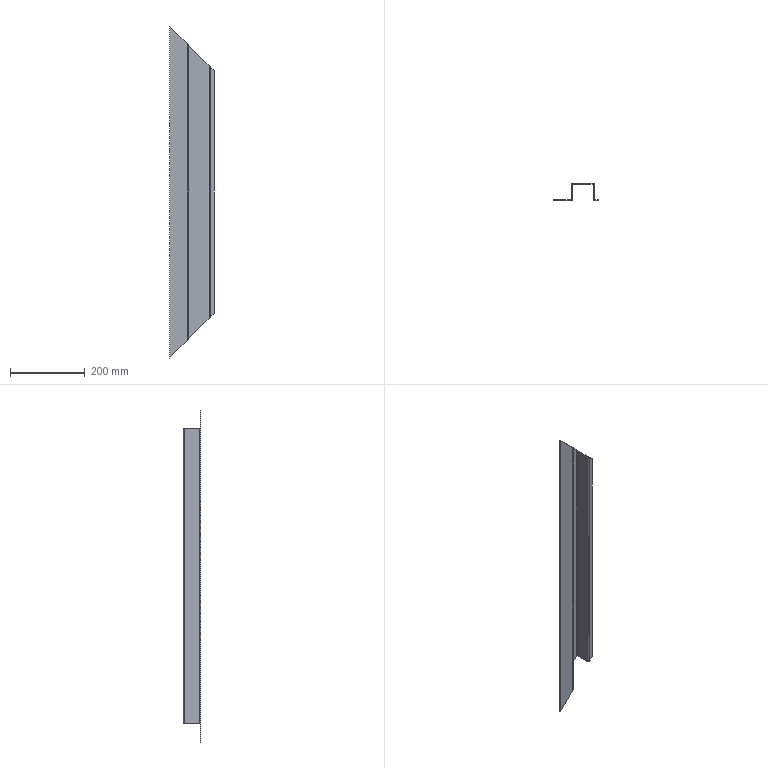Part | STEP file | 750038413 | 1 solid | 38 faces | box 120 x 46.5 x 888 mm | volume 232487 mm3 | plane 22 | cylinder 8 | spline 8 | commonest cylinder face diameters 3 x4 6 x4
STEP:
#1=CARTESIAN_POINT('',(-120.,-1.5,444.));
#2=VERTEX_POINT('',#1);
#3=CARTESIAN_POINT('',(-120.,-1.5,-444.));
#4=VERTEX_POINT('',#3);
#5=CARTESIAN_POINT('',(-120.,-1.5,444.));
#6=DIRECTION('',(0.,0.,-1.));
#7=VECTOR('',#6,1000.);
#8=LINE('',#5,#7);
#9=EDGE_CURVE('',#2,#4,#8,.T.);
#10=ORIENTED_EDGE('',*,*,#9,.T.);
#11=CARTESIAN_POINT('',(-73.,-1.5,-397.));
#12=VERTEX_POINT('',#11);
#13=CARTESIAN_POINT('',(-120.,-1.5,-444.));
#14=DIRECTION('',(0.7071,0.,0.7071));
#15=VECTOR('',#14,1000.);
#16=LINE('',#13,#15);
#17=EDGE_CURVE('',#4,#12,#16,.T.);
#18=ORIENTED_EDGE('',*,*,#17,.T.);
#19=CARTESIAN_POINT('',(-73.,-1.5,397.));
#20=VERTEX_POINT('',#19);
#21=CARTESIAN_POINT('',(-73.,-1.5,444.));
#22=DIRECTION('',(0.,0.,1.));
#23=VECTOR('',#22,1000.);
#24=LINE('',#21,#23);
#25=EDGE_CURVE('',#12,#20,#24,.T.);
#26=ORIENTED_EDGE('',*,*,#25,.T.);
#27=CARTESIAN_POINT('',(-73.,-1.5,397.));
#28=DIRECTION('',(-0.7071,0.,0.7071));
#29=VECTOR('',#28,1000.);
#30=LINE('',#27,#29);
#31=EDGE_CURVE('',#20,#2,#30,.T.);
#32=ORIENTED_EDGE('',*,*,#31,.T.);
#33=EDGE_LOOP('',(#10,#18,#26,#32));
#34=FACE_OUTER_BOUND('',#33,.T.);
#35=CARTESIAN_POINT('',(-71.5,-1.5,444.));
#36=DIRECTION('',(0.,-1.,0.));
#37=DIRECTION('',(1.,0.,0.));
#38=AXIS2_PLACEMENT_3D('',#35,#36,#37);
#39=PLANE('',#38);
#40=ADVANCED_FACE('',(#34),#39,.T.);
#41=CARTESIAN_POINT('',(-73.,0.,-397.));
#42=VERTEX_POINT('',#41);
#43=CARTESIAN_POINT('',(-73.,-0.75,-397.));
#44=DIRECTION('',(0.,-1.,0.));
#45=VECTOR('',#44,1000.);
#46=LINE('',#43,#45);
#47=EDGE_CURVE('',#42,#12,#46,.T.);
#48=ORIENTED_EDGE('',*,*,#47,.T.);
#49=ORIENTED_EDGE('',*,*,#17,.F.);
#50=CARTESIAN_POINT('',(-120.,0.,-444.));
#51=VERTEX_POINT('',#50);
#52=CARTESIAN_POINT('',(-120.,0.,-444.));
#53=DIRECTION('',(0.,1.,0.));
#54=VECTOR('',#53,1000.);
#55=LINE('',#52,#54);
#56=EDGE_CURVE('',#4,#51,#55,.T.);
#57=ORIENTED_EDGE('',*,*,#56,.T.);
#58=CARTESIAN_POINT('',(348.25,0.,24.25));
#59=DIRECTION('',(0.7071,0.,0.7071));
#60=VECTOR('',#59,1000.);
#61=LINE('',#58,#60);
#62=EDGE_CURVE('',#51,#42,#61,.T.);
#63=ORIENTED_EDGE('',*,*,#62,.T.);
#64=EDGE_LOOP('',(#48,#49,#57,#63));
#65=FACE_OUTER_BOUND('',#64,.T.);
#66=CARTESIAN_POINT('',(348.25,0.,24.25));
#67=DIRECTION('',(0.7071,0.,-0.7071));
#68=DIRECTION('',(-0.7071,0.,-0.7071));
#69=AXIS2_PLACEMENT_3D('',#66,#67,#68);
#70=PLANE('',#69);
#71=ADVANCED_FACE('',(#65),#70,.T.);
#72=ORIENTED_EDGE('',*,*,#56,.F.);
#73=ORIENTED_EDGE('',*,*,#9,.F.);
#74=CARTESIAN_POINT('',(-120.,0.,444.));
#75=VERTEX_POINT('',#74);
#76=CARTESIAN_POINT('',(-120.,0.,444.));
#77=DIRECTION('',(0.,1.,0.));
#78=VECTOR('',#77,1000.);
#79=LINE('',#76,#78);
#80=EDGE_CURVE('',#2,#75,#79,.T.);
#81=ORIENTED_EDGE('',*,*,#80,.T.);
#82=CARTESIAN_POINT('',(-120.,0.,444.));
#83=DIRECTION('',(0.,0.,-1.));
#84=VECTOR('',#83,1000.);
#85=LINE('',#82,#84);
#86=EDGE_CURVE('',#75,#51,#85,.T.);
#87=ORIENTED_EDGE('',*,*,#86,.T.);
#88=EDGE_LOOP('',(#72,#73,#81,#87));
#89=FACE_OUTER_BOUND('',#88,.T.);
#90=CARTESIAN_POINT('',(-120.,0.,444.));
#91=DIRECTION('',(-1.,0.,0.));
#92=DIRECTION('',(0.,-1.,0.));
#93=AXIS2_PLACEMENT_3D('',#90,#91,#92);
#94=PLANE('',#93);
#95=ADVANCED_FACE('',(#89),#94,.T.);
#96=ORIENTED_EDGE('',*,*,#80,.F.);
#97=ORIENTED_EDGE('',*,*,#31,.F.);
#98=CARTESIAN_POINT('',(-73.,0.,397.));
#99=VERTEX_POINT('',#98);
#100=CARTESIAN_POINT('',(-73.,-0.75,397.));
#101=DIRECTION('',(0.,1.,0.));
#102=VECTOR('',#101,1000.);
#103=LINE('',#100,#102);
#104=EDGE_CURVE('',#20,#99,#103,.T.);
#105=ORIENTED_EDGE('',*,*,#104,.T.);
#106=CARTESIAN_POINT('',(-95.75,0.,419.75));
#107=DIRECTION('',(-0.7071,0.,0.7071));
#108=VECTOR('',#107,1000.);
#109=LINE('',#106,#108);
#110=EDGE_CURVE('',#99,#75,#109,.T.);
#111=ORIENTED_EDGE('',*,*,#110,.T.);
#112=EDGE_LOOP('',(#96,#97,#105,#111));
#113=FACE_OUTER_BOUND('',#112,.T.);
#114=CARTESIAN_POINT('',(-95.75,0.,419.75));
#115=DIRECTION('',(0.7071,0.,0.7071));
#116=DIRECTION('',(0.7071,0.,-0.7071));
#117=AXIS2_PLACEMENT_3D('',#114,#115,#116);
#118=PLANE('',#117);
#119=ADVANCED_FACE('',(#113),#118,.T.);
#120=ORIENTED_EDGE('',*,*,#25,.F.);
#121=CARTESIAN_POINT('',(-70.,1.5,-394.));
#122=VERTEX_POINT('',#121);
#123=CARTESIAN_POINT('',(-73.,-1.5,-397.));
#124=CARTESIAN_POINT('',(-71.,-1.5,-395.));
#125=CARTESIAN_POINT('',(-70.,0.,-394.));
#126=CARTESIAN_POINT('',(-70.,1.5,-394.));
#127=(BOUNDED_CURVE()B_SPLINE_CURVE(3,(#123,#124,#125,#126),.UNSPECIFIED.,.F.,.F.)B_SPLINE_CURVE_WITH_KNOTS((4,4),(0.,0.005675),.UNSPECIFIED.)CURVE()GEOMETRIC_REPRESENTATION_ITEM()RATIONAL_B_SPLINE_CURVE((0.5,0.5,0.6667,1.))REPRESENTATION_ITEM(''));
#128=EDGE_CURVE('',#12,#122,#127,.T.);
#129=ORIENTED_EDGE('',*,*,#128,.T.);
#130=CARTESIAN_POINT('',(-70.,1.5,394.));
#131=VERTEX_POINT('',#130);
#132=CARTESIAN_POINT('',(-70.,1.5,444.));
#133=DIRECTION('',(0.,0.,1.));
#134=VECTOR('',#133,1000.);
#135=LINE('',#132,#134);
#136=EDGE_CURVE('',#122,#131,#135,.T.);
#137=ORIENTED_EDGE('',*,*,#136,.T.);
#138=CARTESIAN_POINT('',(-70.,1.5,394.));
#139=CARTESIAN_POINT('',(-70.,0.,394.));
#140=CARTESIAN_POINT('',(-71.,-1.5,395.));
#141=CARTESIAN_POINT('',(-73.,-1.5,397.));
#142=(BOUNDED_CURVE()B_SPLINE_CURVE(3,(#138,#139,#140,#141),.UNSPECIFIED.,.F.,.F.)B_SPLINE_CURVE_WITH_KNOTS((4,4),(0.,0.005725),.UNSPECIFIED.)CURVE()GEOMETRIC_REPRESENTATION_ITEM()RATIONAL_B_SPLINE_CURVE((1.,0.6667,0.5,0.5))REPRESENTATION_ITEM(''));
#143=EDGE_CURVE('',#131,#20,#142,.T.);
#144=ORIENTED_EDGE('',*,*,#143,.T.);
#145=EDGE_LOOP('',(#120,#129,#137,#144));
#146=FACE_OUTER_BOUND('',#145,.T.);
#147=CARTESIAN_POINT('',(-73.,1.5,444.));
#148=DIRECTION('',(0.,0.,-1.));
#149=DIRECTION('',(-1.,0.,0.));
#150=AXIS2_PLACEMENT_3D('',#147,#148,#149);
#151=CYLINDRICAL_SURFACE('',#150,3.);
#152=ADVANCED_FACE('',(#146),#151,.T.);
#153=CARTESIAN_POINT('',(-73.,0.,444.));
#154=DIRECTION('',(0.,0.,1.));
#155=VECTOR('',#154,1000.);
#156=LINE('',#153,#155);
#157=EDGE_CURVE('',#42,#99,#156,.T.);
#158=ORIENTED_EDGE('',*,*,#157,.F.);
#159=ORIENTED_EDGE('',*,*,#62,.F.);
#160=ORIENTED_EDGE('',*,*,#86,.F.);
#161=ORIENTED_EDGE('',*,*,#110,.F.);
#162=EDGE_LOOP('',(#158,#159,#160,#161));
#163=FACE_OUTER_BOUND('',#162,.T.);
#164=CARTESIAN_POINT('',(-71.5,0.,444.));
#165=DIRECTION('',(0.,-1.,0.));
#166=DIRECTION('',(1.,0.,0.));
#167=AXIS2_PLACEMENT_3D('',#164,#165,#166);
#168=PLANE('',#167);
#169=ADVANCED_FACE('',(#163),#168,.F.);
#170=ORIENTED_EDGE('',*,*,#128,.F.);
#171=ORIENTED_EDGE('',*,*,#47,.F.);
#172=CARTESIAN_POINT('',(-71.5,1.5,-394.));
#173=VERTEX_POINT('',#172);
#174=CARTESIAN_POINT('',(-71.5,1.5,-394.));
#175=CARTESIAN_POINT('',(-71.5,0.75,-394.));
#176=CARTESIAN_POINT('',(-72.,0.,-395.));
#177=CARTESIAN_POINT('',(-73.,0.,-397.));
#178=(BOUNDED_CURVE()B_SPLINE_CURVE(3,(#174,#175,#176,#177),.UNSPECIFIED.,.F.,.T.)B_SPLINE_CURVE_WITH_KNOTS((4,4),(0.,0.003968),.UNSPECIFIED.)CURVE()GEOMETRIC_REPRESENTATION_ITEM()RATIONAL_B_SPLINE_CURVE((1.,0.6667,0.5,0.5))REPRESENTATION_ITEM(''));
#179=EDGE_CURVE('',#173,#42,#178,.T.);
#180=ORIENTED_EDGE('',*,*,#179,.F.);
#181=CARTESIAN_POINT('',(-70.,1.5,-394.));
#182=DIRECTION('',(-1.,0.,0.));
#183=VECTOR('',#182,1000.);
#184=LINE('',#181,#183);
#185=EDGE_CURVE('',#122,#173,#184,.T.);
#186=ORIENTED_EDGE('',*,*,#185,.F.);
#187=EDGE_LOOP('',(#170,#171,#180,#186));
#188=FACE_OUTER_BOUND('',#187,.T.);
#189=CARTESIAN_POINT('',(-76.,1.5,-400.));
#190=CARTESIAN_POINT('',(-75.5,1.5,-400.));
#191=CARTESIAN_POINT('',(-75.,1.5,-400.));
#192=CARTESIAN_POINT('',(-74.5,1.5,-400.));
#193=CARTESIAN_POINT('',(-76.,-4.5,-400.));
#194=CARTESIAN_POINT('',(-75.5,-3.5,-400.));
#195=CARTESIAN_POINT('',(-75.,-2.5,-400.));
#196=CARTESIAN_POINT('',(-74.5,-1.5,-400.));
#197=CARTESIAN_POINT('',(-70.,-4.5,-394.));
#198=CARTESIAN_POINT('',(-70.5,-3.5,-394.));
#199=CARTESIAN_POINT('',(-71.,-2.5,-394.));
#200=CARTESIAN_POINT('',(-71.5,-1.5,-394.));
#201=CARTESIAN_POINT('',(-70.,1.5,-394.));
#202=CARTESIAN_POINT('',(-70.5,1.5,-394.));
#203=CARTESIAN_POINT('',(-71.,1.5,-394.));
#204=CARTESIAN_POINT('',(-71.5,1.5,-394.));
#205=CARTESIAN_POINT('',(-70.,7.5,-394.));
#206=CARTESIAN_POINT('',(-70.5,6.5,-394.));
#207=CARTESIAN_POINT('',(-71.,5.5,-394.));
#208=CARTESIAN_POINT('',(-71.5,4.5,-394.));
#209=CARTESIAN_POINT('',(-76.,7.5,-400.));
#210=CARTESIAN_POINT('',(-75.5,6.5,-400.));
#211=CARTESIAN_POINT('',(-75.,5.5,-400.));
#212=CARTESIAN_POINT('',(-74.5,4.5,-400.));
#213=CARTESIAN_POINT('',(-76.,1.5,-400.));
#214=CARTESIAN_POINT('',(-75.5,1.5,-400.));
#215=CARTESIAN_POINT('',(-75.,1.5,-400.));
#216=CARTESIAN_POINT('',(-74.5,1.5,-400.));
#217=(BOUNDED_SURFACE()B_SPLINE_SURFACE(3,3,((#189,#190,#191,#192),(#193,#194,#195,#196),(#197,#198,#199,#200),(#201,#202,#203,#204),(#205,#206,#207,#208),(#209,#210,#211,#212),(#213,#214,#215,#216)),.UNSPECIFIED.,.T.,.F.,.F.)B_SPLINE_SURFACE_WITH_KNOTS((4,3,4),(4,4),(0.,0.5,1.),(0.,1.),.UNSPECIFIED.)GEOMETRIC_REPRESENTATION_ITEM()RATIONAL_B_SPLINE_SURFACE(((1.,1.,1.,1.),(0.3333,0.3333,0.3333,0.3333),(0.3333,0.3333,0.3333,0.3333),(1.,1.,1.,1.),(0.3333,0.3333,0.3333,0.3333),(0.3333,0.3333,0.3333,0.3333),(1.,1.,1.,1.)))REPRESENTATION_ITEM('')SURFACE());
#218=ADVANCED_FACE('',(#188),#217,.F.);
#219=ORIENTED_EDGE('',*,*,#104,.F.);
#220=ORIENTED_EDGE('',*,*,#143,.F.);
#221=CARTESIAN_POINT('',(-71.5,1.5,394.));
#222=VERTEX_POINT('',#221);
#223=CARTESIAN_POINT('',(-70.,1.5,394.));
#224=DIRECTION('',(1.,0.,0.));
#225=VECTOR('',#224,1000.);
#226=LINE('',#223,#225);
#227=EDGE_CURVE('',#222,#131,#226,.T.);
#228=ORIENTED_EDGE('',*,*,#227,.F.);
#229=CARTESIAN_POINT('',(-73.,0.,397.));
#230=CARTESIAN_POINT('',(-72.,0.,395.));
#231=CARTESIAN_POINT('',(-71.5,0.75,394.));
#232=CARTESIAN_POINT('',(-71.5,1.5,394.));
#233=(BOUNDED_CURVE()B_SPLINE_CURVE(3,(#229,#230,#231,#232),.UNSPECIFIED.,.F.,.F.)B_SPLINE_CURVE_WITH_KNOTS((4,4),(0.,0.003921),.UNSPECIFIED.)CURVE()GEOMETRIC_REPRESENTATION_ITEM()RATIONAL_B_SPLINE_CURVE((0.5,0.5,0.6667,1.))REPRESENTATION_ITEM(''));
#234=EDGE_CURVE('',#99,#222,#233,.T.);
#235=ORIENTED_EDGE('',*,*,#234,.F.);
#236=EDGE_LOOP('',(#219,#220,#228,#235));
#237=FACE_OUTER_BOUND('',#236,.T.);
#238=CARTESIAN_POINT('',(-70.,1.5,394.));
#239=CARTESIAN_POINT('',(-70.5,1.5,394.));
#240=CARTESIAN_POINT('',(-71.,1.5,394.));
#241=CARTESIAN_POINT('',(-71.5,1.5,394.));
#242=CARTESIAN_POINT('',(-70.,-4.5,394.));
#243=CARTESIAN_POINT('',(-70.5,-3.5,394.));
#244=CARTESIAN_POINT('',(-71.,-2.5,394.));
#245=CARTESIAN_POINT('',(-71.5,-1.5,394.));
#246=CARTESIAN_POINT('',(-76.,-4.5,400.));
#247=CARTESIAN_POINT('',(-75.5,-3.5,400.));
#248=CARTESIAN_POINT('',(-75.,-2.5,400.));
#249=CARTESIAN_POINT('',(-74.5,-1.5,400.));
#250=CARTESIAN_POINT('',(-76.,1.5,400.));
#251=CARTESIAN_POINT('',(-75.5,1.5,400.));
#252=CARTESIAN_POINT('',(-75.,1.5,400.));
#253=CARTESIAN_POINT('',(-74.5,1.5,400.));
#254=CARTESIAN_POINT('',(-76.,7.5,400.));
#255=CARTESIAN_POINT('',(-75.5,6.5,400.));
#256=CARTESIAN_POINT('',(-75.,5.5,400.));
#257=CARTESIAN_POINT('',(-74.5,4.5,400.));
#258=CARTESIAN_POINT('',(-70.,7.5,394.));
#259=CARTESIAN_POINT('',(-70.5,6.5,394.));
#260=CARTESIAN_POINT('',(-71.,5.5,394.));
#261=CARTESIAN_POINT('',(-71.5,4.5,394.));
#262=CARTESIAN_POINT('',(-70.,1.5,394.));
#263=CARTESIAN_POINT('',(-70.5,1.5,394.));
#264=CARTESIAN_POINT('',(-71.,1.5,394.));
#265=CARTESIAN_POINT('',(-71.5,1.5,394.));
#266=(BOUNDED_SURFACE()B_SPLINE_SURFACE(3,3,((#238,#239,#240,#241),(#242,#243,#244,#245),(#246,#247,#248,#249),(#250,#251,#252,#253),(#254,#255,#256,#257),(#258,#259,#260,#261),(#262,#263,#264,#265)),.UNSPECIFIED.,.T.,.F.,.F.)B_SPLINE_SURFACE_WITH_KNOTS((4,3,4),(4,4),(0.,0.5,1.),(0.,1.),.UNSPECIFIED.)GEOMETRIC_REPRESENTATION_ITEM()RATIONAL_B_SPLINE_SURFACE(((1.,1.,1.,1.),(0.3333,0.3333,0.3333,0.3333),(0.3333,0.3333,0.3333,0.3333),(1.,1.,1.,1.),(0.3333,0.3333,0.3333,0.3333),(0.3333,0.3333,0.3333,0.3333),(1.,1.,1.,1.)))REPRESENTATION_ITEM('')SURFACE());
#267=ADVANCED_FACE('',(#237),#266,.F.);
#268=ORIENTED_EDGE('',*,*,#136,.F.);
#269=CARTESIAN_POINT('',(-70.,42.,-394.));
#270=VERTEX_POINT('',#269);
#271=CARTESIAN_POINT('',(-70.,45.,-394.));
#272=DIRECTION('',(0.,1.,0.));
#273=VECTOR('',#272,1000.);
#274=LINE('',#271,#273);
#275=EDGE_CURVE('',#122,#270,#274,.T.);
#276=ORIENTED_EDGE('',*,*,#275,.T.);
#277=CARTESIAN_POINT('',(-70.,42.,394.));
#278=VERTEX_POINT('',#277);
#279=CARTESIAN_POINT('',(-70.,42.,444.));
#280=DIRECTION('',(0.,0.,1.));
#281=VECTOR('',#280,1000.);
#282=LINE('',#279,#281);
#283=EDGE_CURVE('',#270,#278,#282,.T.);
#284=ORIENTED_EDGE('',*,*,#283,.T.);
#285=CARTESIAN_POINT('',(-70.,45.,394.));
#286=DIRECTION('',(0.,-1.,0.));
#287=VECTOR('',#286,1000.);
#288=LINE('',#285,#287);
#289=EDGE_CURVE('',#278,#131,#288,.T.);
#290=ORIENTED_EDGE('',*,*,#289,.T.);
#291=EDGE_LOOP('',(#268,#276,#284,#290));
#292=FACE_OUTER_BOUND('',#291,.T.);
#293=CARTESIAN_POINT('',(-70.,45.,444.));
#294=DIRECTION('',(1.,0.,0.));
#295=DIRECTION('',(0.,0.,-1.));
#296=AXIS2_PLACEMENT_3D('',#293,#294,#295);
#297=PLANE('',#296);
#298=ADVANCED_FACE('',(#292),#297,.T.);
#299=CARTESIAN_POINT('',(-71.5,1.5,444.));
#300=DIRECTION('',(0.,0.,1.));
#301=VECTOR('',#300,1000.);
#302=LINE('',#299,#301);
#303=EDGE_CURVE('',#173,#222,#302,.T.);
#304=ORIENTED_EDGE('',*,*,#303,.F.);
#305=ORIENTED_EDGE('',*,*,#179,.T.);
#306=ORIENTED_EDGE('',*,*,#157,.T.);
#307=ORIENTED_EDGE('',*,*,#234,.T.);
#308=EDGE_LOOP('',(#304,#305,#306,#307));
#309=FACE_OUTER_BOUND('',#308,.T.);
#310=CARTESIAN_POINT('',(-73.,1.5,444.));
#311=DIRECTION('',(0.,0.,-1.));
#312=DIRECTION('',(-1.,0.,0.));
#313=AXIS2_PLACEMENT_3D('',#310,#311,#312);
#314=CYLINDRICAL_SURFACE('',#313,1.5);
#315=ADVANCED_FACE('',(#309),#314,.F.);
#316=ORIENTED_EDGE('',*,*,#185,.T.);
#317=CARTESIAN_POINT('',(-71.5,42.,-394.));
#318=VERTEX_POINT('',#317);
#319=CARTESIAN_POINT('',(-71.5,45.,-394.));
#320=DIRECTION('',(0.,1.,0.));
#321=VECTOR('',#320,1000.);
#322=LINE('',#319,#321);
#323=EDGE_CURVE('',#173,#318,#322,.T.);
#324=ORIENTED_EDGE('',*,*,#323,.T.);
#325=CARTESIAN_POINT('',(-70.75,42.,-394.));
#326=DIRECTION('',(1.,0.,0.));
#327=VECTOR('',#326,1000.);
#328=LINE('',#325,#327);
#329=EDGE_CURVE('',#318,#270,#328,.T.);
#330=ORIENTED_EDGE('',*,*,#329,.T.);
#331=ORIENTED_EDGE('',*,*,#275,.F.);
#332=EDGE_LOOP('',(#316,#324,#330,#331));
#333=FACE_OUTER_BOUND('',#332,.T.);
#334=CARTESIAN_POINT('',(-70.,45.,-394.));
#335=DIRECTION('',(0.,0.,-1.));
#336=DIRECTION('',(-1.,0.,0.));
#337=AXIS2_PLACEMENT_3D('',#334,#335,#336);
#338=PLANE('',#337);
#339=ADVANCED_FACE('',(#333),#338,.T.);
#340=CARTESIAN_POINT('',(-71.5,42.,394.));
#341=VERTEX_POINT('',#340);
#342=CARTESIAN_POINT('',(-70.75,42.,394.));
#343=DIRECTION('',(-1.,0.,0.));
#344=VECTOR('',#343,1000.);
#345=LINE('',#342,#344);
#346=EDGE_CURVE('',#278,#341,#345,.T.);
#347=ORIENTED_EDGE('',*,*,#346,.T.);
#348=CARTESIAN_POINT('',(-71.5,45.,394.));
#349=DIRECTION('',(0.,-1.,0.));
#350=VECTOR('',#349,1000.);
#351=LINE('',#348,#350);
#352=EDGE_CURVE('',#341,#222,#351,.T.);
#353=ORIENTED_EDGE('',*,*,#352,.T.);
#354=ORIENTED_EDGE('',*,*,#227,.T.);
#355=ORIENTED_EDGE('',*,*,#289,.F.);
#356=EDGE_LOOP('',(#347,#353,#354,#355));
#357=FACE_OUTER_BOUND('',#356,.T.);
#358=CARTESIAN_POINT('',(-70.,45.,394.));
#359=DIRECTION('',(0.,0.,1.));
#360=DIRECTION('',(1.,0.,0.));
#361=AXIS2_PLACEMENT_3D('',#358,#359,#360);
#362=PLANE('',#361);
#363=ADVANCED_FACE('',(#357),#362,.T.);
#364=CARTESIAN_POINT('',(-68.5,43.5,392.5));
#365=VERTEX_POINT('',#364);
#366=CARTESIAN_POINT('',(-70.,42.,394.));
#367=CARTESIAN_POINT('',(-70.,42.75,394.));
#368=CARTESIAN_POINT('',(-69.5,43.5,393.5));
#369=CARTESIAN_POINT('',(-68.5,43.5,392.5));
#370=(BOUNDED_CURVE()B_SPLINE_CURVE(3,(#366,#367,#368,#369),.UNSPECIFIED.,.F.,.T.)B_SPLINE_CURVE_WITH_KNOTS((4,4),(0.,0.002854),.UNSPECIFIED.)CURVE()GEOMETRIC_REPRESENTATION_ITEM()RATIONAL_B_SPLINE_CURVE((1.,0.6667,0.5,0.5))REPRESENTATION_ITEM(''));
#371=EDGE_CURVE('',#278,#365,#370,.T.);
#372=ORIENTED_EDGE('',*,*,#371,.F.);
#373=ORIENTED_EDGE('',*,*,#283,.F.);
#374=CARTESIAN_POINT('',(-68.5,43.5,-392.5));
#375=VERTEX_POINT('',#374);
#376=CARTESIAN_POINT('',(-68.5,43.5,-392.5));
#377=CARTESIAN_POINT('',(-69.5,43.5,-393.5));
#378=CARTESIAN_POINT('',(-70.,42.75,-394.));
#379=CARTESIAN_POINT('',(-70.,42.,-394.));
#380=(BOUNDED_CURVE()B_SPLINE_CURVE(3,(#376,#377,#378,#379),.UNSPECIFIED.,.F.,.F.)B_SPLINE_CURVE_WITH_KNOTS((4,4),(0.,0.002839),.UNSPECIFIED.)CURVE()GEOMETRIC_REPRESENTATION_ITEM()RATIONAL_B_SPLINE_CURVE((0.5,0.5,0.6667,1.))REPRESENTATION_ITEM(''));
#381=EDGE_CURVE('',#375,#270,#380,.T.);
#382=ORIENTED_EDGE('',*,*,#381,.F.);
#383=CARTESIAN_POINT('',(-68.5,43.5,444.));
#384=DIRECTION('',(0.,0.,-1.));
#385=VECTOR('',#384,1000.);
#386=LINE('',#383,#385);
#387=EDGE_CURVE('',#365,#375,#386,.T.);
#388=ORIENTED_EDGE('',*,*,#387,.F.);
#389=EDGE_LOOP('',(#372,#373,#382,#388));
#390=FACE_OUTER_BOUND('',#389,.T.);
#391=CARTESIAN_POINT('',(-68.5,42.,444.));
#392=DIRECTION('',(0.,0.,-1.));
#393=DIRECTION('',(-1.,0.,0.));
#394=AXIS2_PLACEMENT_3D('',#391,#392,#393);
#395=CYLINDRICAL_SURFACE('',#394,1.5);
#396=ADVANCED_FACE('',(#390),#395,.F.);
#397=CARTESIAN_POINT('',(-71.5,42.,444.));
#398=DIRECTION('',(0.,0.,1.));
#399=VECTOR('',#398,1000.);
#400=LINE('',#397,#399);
#401=EDGE_CURVE('',#318,#341,#400,.T.);
#402=ORIENTED_EDGE('',*,*,#401,.F.);
#403=ORIENTED_EDGE('',*,*,#323,.F.);
#404=ORIENTED_EDGE('',*,*,#303,.T.);
#405=ORIENTED_EDGE('',*,*,#352,.F.);
#406=EDGE_LOOP('',(#402,#403,#404,#405));
#407=FACE_OUTER_BOUND('',#406,.T.);
#408=CARTESIAN_POINT('',(-71.5,45.,444.));
#409=DIRECTION('',(1.,0.,0.));
#410=DIRECTION('',(0.,0.,-1.));
#411=AXIS2_PLACEMENT_3D('',#408,#409,#410);
#412=PLANE('',#411);
#413=ADVANCED_FACE('',(#407),#412,.F.);
#414=ORIENTED_EDGE('',*,*,#387,.T.);
#415=CARTESIAN_POINT('',(-14.5,43.5,-338.5));
#416=VERTEX_POINT('',#415);
#417=CARTESIAN_POINT('',(-68.5,43.5,-392.5));
#418=DIRECTION('',(0.7071,0.,0.7071));
#419=VECTOR('',#418,1000.);
#420=LINE('',#417,#419);
#421=EDGE_CURVE('',#375,#416,#420,.T.);
#422=ORIENTED_EDGE('',*,*,#421,.T.);
#423=CARTESIAN_POINT('',(-14.5,43.5,338.5));
#424=VERTEX_POINT('',#423);
#425=CARTESIAN_POINT('',(-14.5,43.5,444.));
#426=DIRECTION('',(0.,0.,1.));
#427=VECTOR('',#426,1000.);
#428=LINE('',#425,#427);
#429=EDGE_CURVE('',#416,#424,#428,.T.);
#430=ORIENTED_EDGE('',*,*,#429,.T.);
#431=CARTESIAN_POINT('',(-14.5,43.5,338.5));
#432=DIRECTION('',(-0.7071,0.,0.7071));
#433=VECTOR('',#432,1000.);
#434=LINE('',#431,#433);
#435=EDGE_CURVE('',#424,#365,#434,.T.);
#436=ORIENTED_EDGE('',*,*,#435,.T.);
#437=EDGE_LOOP('',(#414,#422,#430,#436));
#438=FACE_OUTER_BOUND('',#437,.T.);
#439=CARTESIAN_POINT('',(-11.5,43.5,444.));
#440=DIRECTION('',(0.,-1.,0.));
#441=DIRECTION('',(1.,0.,0.));
#442=AXIS2_PLACEMENT_3D('',#439,#440,#441);
#443=PLANE('',#442);
#444=ADVANCED_FACE('',(#438),#443,.T.);
#445=ORIENTED_EDGE('',*,*,#371,.T.);
#446=CARTESIAN_POINT('',(-68.5,45.,392.5));
#447=VERTEX_POINT('',#446);
#448=CARTESIAN_POINT('',(-68.5,44.25,392.5));
#449=DIRECTION('',(0.,-1.,0.));
#450=VECTOR('',#449,1000.);
#451=LINE('',#448,#450);
#452=EDGE_CURVE('',#447,#365,#451,.T.);
#453=ORIENTED_EDGE('',*,*,#452,.F.);
#454=CARTESIAN_POINT('',(-71.5,42.,394.));
#455=CARTESIAN_POINT('',(-71.5,43.5,394.));
#456=CARTESIAN_POINT('',(-70.5,45.,393.5));
#457=CARTESIAN_POINT('',(-68.5,45.,392.5));
#458=(BOUNDED_CURVE()B_SPLINE_CURVE(3,(#454,#455,#456,#457),.UNSPECIFIED.,.F.,.T.)B_SPLINE_CURVE_WITH_KNOTS((4,4),(0.,0.00499),.UNSPECIFIED.)CURVE()GEOMETRIC_REPRESENTATION_ITEM()RATIONAL_B_SPLINE_CURVE((1.,0.6667,0.5,0.5))REPRESENTATION_ITEM(''));
#459=EDGE_CURVE('',#341,#447,#458,.T.);
#460=ORIENTED_EDGE('',*,*,#459,.F.);
#461=ORIENTED_EDGE('',*,*,#346,.F.);
#462=EDGE_LOOP('',(#445,#453,#460,#461));
#463=FACE_OUTER_BOUND('',#462,.T.);
#464=CARTESIAN_POINT('',(-67.,42.,391.));
#465=CARTESIAN_POINT('',(-66.5,42.,391.));
#466=CARTESIAN_POINT('',(-66.,42.,391.));
#467=CARTESIAN_POINT('',(-65.5,42.,391.));
#468=CARTESIAN_POINT('',(-67.,45.,391.));
#469=CARTESIAN_POINT('',(-66.5,46.,391.));
#470=CARTESIAN_POINT('',(-66.,47.,391.));
#471=CARTESIAN_POINT('',(-65.5,48.,391.));
#472=CARTESIAN_POINT('',(-70.,45.,394.));
#473=CARTESIAN_POINT('',(-70.5,46.,394.));
#474=CARTESIAN_POINT('',(-71.,47.,394.));
#475=CARTESIAN_POINT('',(-71.5,48.,394.));
#476=CARTESIAN_POINT('',(-70.,42.,394.));
#477=CARTESIAN_POINT('',(-70.5,42.,394.));
#478=CARTESIAN_POINT('',(-71.,42.,394.));
#479=CARTESIAN_POINT('',(-71.5,42.,394.));
#480=CARTESIAN_POINT('',(-70.,39.,394.));
#481=CARTESIAN_POINT('',(-70.5,38.,394.));
#482=CARTESIAN_POINT('',(-71.,37.,394.));
#483=CARTESIAN_POINT('',(-71.5,36.,394.));
#484=CARTESIAN_POINT('',(-67.,39.,391.));
#485=CARTESIAN_POINT('',(-66.5,38.,391.));
#486=CARTESIAN_POINT('',(-66.,37.,391.));
#487=CARTESIAN_POINT('',(-65.5,36.,391.));
#488=CARTESIAN_POINT('',(-67.,42.,391.));
#489=CARTESIAN_POINT('',(-66.5,42.,391.));
#490=CARTESIAN_POINT('',(-66.,42.,391.));
#491=CARTESIAN_POINT('',(-65.5,42.,391.));
#492=(BOUNDED_SURFACE()B_SPLINE_SURFACE(3,3,((#464,#465,#466,#467),(#468,#469,#470,#471),(#472,#473,#474,#475),(#476,#477,#478,#479),(#480,#481,#482,#483),(#484,#485,#486,#487),(#488,#489,#490,#491)),.UNSPECIFIED.,.T.,.F.,.F.)B_SPLINE_SURFACE_WITH_KNOTS((4,3,4),(4,4),(0.,0.5,1.),(0.,1.),.UNSPECIFIED.)GEOMETRIC_REPRESENTATION_ITEM()RATIONAL_B_SPLINE_SURFACE(((1.,1.,1.,1.),(0.3333,0.3333,0.3333,0.3333),(0.3333,0.3333,0.3333,0.3333),(1.,1.,1.,1.),(0.3333,0.3333,0.3333,0.3333),(0.3333,0.3333,0.3333,0.3333),(1.,1.,1.,1.)))REPRESENTATION_ITEM('')SURFACE());
#493=ADVANCED_FACE('',(#463),#492,.F.);
#494=ORIENTED_EDGE('',*,*,#381,.T.);
#495=ORIENTED_EDGE('',*,*,#329,.F.);
#496=CARTESIAN_POINT('',(-68.5,45.,-392.5));
#497=VERTEX_POINT('',#496);
#498=CARTESIAN_POINT('',(-68.5,45.,-392.5));
#499=CARTESIAN_POINT('',(-70.5,45.,-393.5));
#500=CARTESIAN_POINT('',(-71.5,43.5,-394.));
#501=CARTESIAN_POINT('',(-71.5,42.,-394.));
#502=(BOUNDED_CURVE()B_SPLINE_CURVE(3,(#498,#499,#500,#501),.UNSPECIFIED.,.F.,.F.)B_SPLINE_CURVE_WITH_KNOTS((4,4),(0.,0.004967),.UNSPECIFIED.)CURVE()GEOMETRIC_REPRESENTATION_ITEM()RATIONAL_B_SPLINE_CURVE((0.5,0.5,0.6667,1.))REPRESENTATION_ITEM(''));
#503=EDGE_CURVE('',#497,#318,#502,.T.);
#504=ORIENTED_EDGE('',*,*,#503,.F.);
#505=CARTESIAN_POINT('',(-68.5,44.25,-392.5));
#506=DIRECTION('',(0.,1.,0.));
#507=VECTOR('',#506,1000.);
#508=LINE('',#505,#507);
#509=EDGE_CURVE('',#375,#497,#508,.T.);
#510=ORIENTED_EDGE('',*,*,#509,.F.);
#511=EDGE_LOOP('',(#494,#495,#504,#510));
#512=FACE_OUTER_BOUND('',#511,.T.);
#513=CARTESIAN_POINT('',(-70.,42.,-394.));
#514=CARTESIAN_POINT('',(-70.5,42.,-394.));
#515=CARTESIAN_POINT('',(-71.,42.,-394.));
#516=CARTESIAN_POINT('',(-71.5,42.,-394.));
#517=CARTESIAN_POINT('',(-70.,45.,-394.));
#518=CARTESIAN_POINT('',(-70.5,46.,-394.));
#519=CARTESIAN_POINT('',(-71.,47.,-394.));
#520=CARTESIAN_POINT('',(-71.5,48.,-394.));
#521=CARTESIAN_POINT('',(-67.,45.,-391.));
#522=CARTESIAN_POINT('',(-66.5,46.,-391.));
#523=CARTESIAN_POINT('',(-66.,47.,-391.));
#524=CARTESIAN_POINT('',(-65.5,48.,-391.));
#525=CARTESIAN_POINT('',(-67.,42.,-391.));
#526=CARTESIAN_POINT('',(-66.5,42.,-391.));
#527=CARTESIAN_POINT('',(-66.,42.,-391.));
#528=CARTESIAN_POINT('',(-65.5,42.,-391.));
#529=CARTESIAN_POINT('',(-67.,39.,-391.));
#530=CARTESIAN_POINT('',(-66.5,38.,-391.));
#531=CARTESIAN_POINT('',(-66.,37.,-391.));
#532=CARTESIAN_POINT('',(-65.5,36.,-391.));
#533=CARTESIAN_POINT('',(-70.,39.,-394.));
#534=CARTESIAN_POINT('',(-70.5,38.,-394.));
#535=CARTESIAN_POINT('',(-71.,37.,-394.));
#536=CARTESIAN_POINT('',(-71.5,36.,-394.));
#537=CARTESIAN_POINT('',(-70.,42.,-394.));
#538=CARTESIAN_POINT('',(-70.5,42.,-394.));
#539=CARTESIAN_POINT('',(-71.,42.,-394.));
#540=CARTESIAN_POINT('',(-71.5,42.,-394.));
#541=(BOUNDED_SURFACE()B_SPLINE_SURFACE(3,3,((#513,#514,#515,#516),(#517,#518,#519,#520),(#521,#522,#523,#524),(#525,#526,#527,#528),(#529,#530,#531,#532),(#533,#534,#535,#536),(#537,#538,#539,#540)),.UNSPECIFIED.,.T.,.F.,.F.)B_SPLINE_SURFACE_WITH_KNOTS((4,3,4),(4,4),(0.,0.5,1.),(0.,1.),.UNSPECIFIED.)GEOMETRIC_REPRESENTATION_ITEM()RATIONAL_B_SPLINE_SURFACE(((1.,1.,1.,1.),(0.3333,0.3333,0.3333,0.3333),(0.3333,0.3333,0.3333,0.3333),(1.,1.,1.,1.),(0.3333,0.3333,0.3333,0.3333),(0.3333,0.3333,0.3333,0.3333),(1.,1.,1.,1.)))REPRESENTATION_ITEM('')SURFACE());
#542=ADVANCED_FACE('',(#512),#541,.F.);
#543=ORIENTED_EDGE('',*,*,#503,.T.);
#544=ORIENTED_EDGE('',*,*,#401,.T.);
#545=ORIENTED_EDGE('',*,*,#459,.T.);
#546=CARTESIAN_POINT('',(-68.5,45.,444.));
#547=DIRECTION('',(0.,0.,-1.));
#548=VECTOR('',#547,1000.);
#549=LINE('',#546,#548);
#550=EDGE_CURVE('',#447,#497,#549,.T.);
#551=ORIENTED_EDGE('',*,*,#550,.T.);
#552=EDGE_LOOP('',(#543,#544,#545,#551));
#553=FACE_OUTER_BOUND('',#552,.T.);
#554=CARTESIAN_POINT('',(-68.5,42.,444.));
#555=DIRECTION('',(0.,0.,-1.));
#556=DIRECTION('',(-1.,0.,0.));
#557=AXIS2_PLACEMENT_3D('',#554,#555,#556);
#558=CYLINDRICAL_SURFACE('',#557,3.);
#559=ADVANCED_FACE('',(#553),#558,.T.);
#560=CARTESIAN_POINT('',(-14.5,45.,-338.5));
#561=VERTEX_POINT('',#560);
#562=CARTESIAN_POINT('',(-14.5,44.25,-338.5));
#563=DIRECTION('',(0.,-1.,0.));
#564=VECTOR('',#563,1000.);
#565=LINE('',#562,#564);
#566=EDGE_CURVE('',#561,#416,#565,.T.);
#567=ORIENTED_EDGE('',*,*,#566,.T.);
#568=ORIENTED_EDGE('',*,*,#421,.F.);
#569=ORIENTED_EDGE('',*,*,#509,.T.);
#570=CARTESIAN_POINT('',(378.25,45.,54.25));
#571=DIRECTION('',(0.7071,0.,0.7071));
#572=VECTOR('',#571,1000.);
#573=LINE('',#570,#572);
#574=EDGE_CURVE('',#497,#561,#573,.T.);
#575=ORIENTED_EDGE('',*,*,#574,.T.);
#576=EDGE_LOOP('',(#567,#568,#569,#575));
#577=FACE_OUTER_BOUND('',#576,.T.);
#578=CARTESIAN_POINT('',(378.25,45.,54.25));
#579=DIRECTION('',(0.7071,0.,-0.7071));
#580=DIRECTION('',(-0.7071,0.,-0.7071));
#581=AXIS2_PLACEMENT_3D('',#578,#579,#580);
#582=PLANE('',#581);
#583=ADVANCED_FACE('',(#577),#582,.T.);
#584=ORIENTED_EDGE('',*,*,#452,.T.);
#585=ORIENTED_EDGE('',*,*,#435,.F.);
#586=CARTESIAN_POINT('',(-14.5,45.,338.5));
#587=VERTEX_POINT('',#586);
#588=CARTESIAN_POINT('',(-14.5,44.25,338.5));
#589=DIRECTION('',(0.,1.,0.));
#590=VECTOR('',#589,1000.);
#591=LINE('',#588,#590);
#592=EDGE_CURVE('',#424,#587,#591,.T.);
#593=ORIENTED_EDGE('',*,*,#592,.T.);
#594=CARTESIAN_POINT('',(-65.75,45.,389.75));
#595=DIRECTION('',(-0.7071,0.,0.7071));
#596=VECTOR('',#595,1000.);
#597=LINE('',#594,#596);
#598=EDGE_CURVE('',#587,#447,#597,.T.);
#599=ORIENTED_EDGE('',*,*,#598,.T.);
#600=EDGE_LOOP('',(#584,#585,#593,#599));
#601=FACE_OUTER_BOUND('',#600,.T.);
#602=CARTESIAN_POINT('',(-65.75,45.,389.75));
#603=DIRECTION('',(0.7071,0.,0.7071));
#604=DIRECTION('',(0.7071,0.,-0.7071));
#605=AXIS2_PLACEMENT_3D('',#602,#603,#604);
#606=PLANE('',#605);
#607=ADVANCED_FACE('',(#601),#606,.T.);
#608=CARTESIAN_POINT('',(-13.,42.,335.5));
#609=VERTEX_POINT('',#608);
#610=CARTESIAN_POINT('',(-14.5,43.5,338.5));
#611=CARTESIAN_POINT('',(-13.5,43.5,336.5));
#612=CARTESIAN_POINT('',(-13.,42.75,335.5));
#613=CARTESIAN_POINT('',(-13.,42.,335.5));
#614=(BOUNDED_CURVE()B_SPLINE_CURVE(3,(#610,#611,#612,#613),.UNSPECIFIED.,.F.,.F.)B_SPLINE_CURVE_WITH_KNOTS((4,4),(0.,0.003921),.UNSPECIFIED.)CURVE()GEOMETRIC_REPRESENTATION_ITEM()RATIONAL_B_SPLINE_CURVE((0.5,0.5,0.6667,1.))REPRESENTATION_ITEM(''));
#615=EDGE_CURVE('',#424,#609,#614,.T.);
#616=ORIENTED_EDGE('',*,*,#615,.F.);
#617=ORIENTED_EDGE('',*,*,#429,.F.);
#618=CARTESIAN_POINT('',(-13.,42.,-335.5));
#619=VERTEX_POINT('',#618);
#620=CARTESIAN_POINT('',(-13.,42.,-335.5));
#621=CARTESIAN_POINT('',(-13.,42.75,-335.5));
#622=CARTESIAN_POINT('',(-13.5,43.5,-336.5));
#623=CARTESIAN_POINT('',(-14.5,43.5,-338.5));
#624=(BOUNDED_CURVE()B_SPLINE_CURVE(3,(#620,#621,#622,#623),.UNSPECIFIED.,.F.,.F.)B_SPLINE_CURVE_WITH_KNOTS((4,4),(0.,0.003968),.UNSPECIFIED.)CURVE()GEOMETRIC_REPRESENTATION_ITEM()RATIONAL_B_SPLINE_CURVE((1.,0.6667,0.5,0.5))REPRESENTATION_ITEM(''));
#625=EDGE_CURVE('',#619,#416,#624,.T.);
#626=ORIENTED_EDGE('',*,*,#625,.F.);
#627=CARTESIAN_POINT('',(-13.,42.,444.));
#628=DIRECTION('',(0.,0.,-1.));
#629=VECTOR('',#628,1000.);
#630=LINE('',#627,#629);
#631=EDGE_CURVE('',#609,#619,#630,.T.);
#632=ORIENTED_EDGE('',*,*,#631,.F.);
#633=EDGE_LOOP('',(#616,#617,#626,#632));
#634=FACE_OUTER_BOUND('',#633,.T.);
#635=CARTESIAN_POINT('',(-14.5,42.,444.));
#636=DIRECTION('',(0.,0.,-1.));
#637=DIRECTION('',(-1.,0.,0.));
#638=AXIS2_PLACEMENT_3D('',#635,#636,#637);
#639=CYLINDRICAL_SURFACE('',#638,1.5);
#640=ADVANCED_FACE('',(#634),#639,.F.);
#641=CARTESIAN_POINT('',(-14.5,45.,444.));
#642=DIRECTION('',(0.,0.,1.));
#643=VECTOR('',#642,1000.);
#644=LINE('',#641,#643);
#645=EDGE_CURVE('',#561,#587,#644,.T.);
#646=ORIENTED_EDGE('',*,*,#645,.F.);
#647=ORIENTED_EDGE('',*,*,#574,.F.);
#648=ORIENTED_EDGE('',*,*,#550,.F.);
#649=ORIENTED_EDGE('',*,*,#598,.F.);
#650=EDGE_LOOP('',(#646,#647,#648,#649));
#651=FACE_OUTER_BOUND('',#650,.T.);
#652=CARTESIAN_POINT('',(-11.5,45.,444.));
#653=DIRECTION('',(0.,-1.,0.));
#654=DIRECTION('',(1.,0.,0.));
#655=AXIS2_PLACEMENT_3D('',#652,#653,#654);
#656=PLANE('',#655);
#657=ADVANCED_FACE('',(#651),#656,.F.);
#658=ORIENTED_EDGE('',*,*,#631,.T.);
#659=CARTESIAN_POINT('',(-13.,1.5,-335.5));
#660=VERTEX_POINT('',#659);
#661=CARTESIAN_POINT('',(-13.,0.,-335.5));
#662=DIRECTION('',(0.,-1.,0.));
#663=VECTOR('',#662,1000.);
#664=LINE('',#661,#663);
#665=EDGE_CURVE('',#619,#660,#664,.T.);
#666=ORIENTED_EDGE('',*,*,#665,.T.);
#667=CARTESIAN_POINT('',(-13.,1.5,335.5));
#668=VERTEX_POINT('',#667);
#669=CARTESIAN_POINT('',(-13.,1.5,444.));
#670=DIRECTION('',(0.,0.,1.));
#671=VECTOR('',#670,1000.);
#672=LINE('',#669,#671);
#673=EDGE_CURVE('',#660,#668,#672,.T.);
#674=ORIENTED_EDGE('',*,*,#673,.T.);
#675=CARTESIAN_POINT('',(-13.,0.,335.5));
#676=DIRECTION('',(0.,1.,0.));
#677=VECTOR('',#676,1000.);
#678=LINE('',#675,#677);
#679=EDGE_CURVE('',#668,#609,#678,.T.);
#680=ORIENTED_EDGE('',*,*,#679,.T.);
#681=EDGE_LOOP('',(#658,#666,#674,#680));
#682=FACE_OUTER_BOUND('',#681,.T.);
#683=CARTESIAN_POINT('',(-13.,0.,444.));
#684=DIRECTION('',(-1.,0.,0.));
#685=DIRECTION('',(0.,0.,1.));
#686=AXIS2_PLACEMENT_3D('',#683,#684,#685);
#687=PLANE('',#686);
#688=ADVANCED_FACE('',(#682),#687,.T.);
#689=CARTESIAN_POINT('',(-11.5,42.,335.5));
#690=VERTEX_POINT('',#689);
#691=CARTESIAN_POINT('',(-14.5,45.,338.5));
#692=CARTESIAN_POINT('',(-12.5,45.,336.5));
#693=CARTESIAN_POINT('',(-11.5,43.5,335.5));
#694=CARTESIAN_POINT('',(-11.5,42.,335.5));
#695=(BOUNDED_CURVE()B_SPLINE_CURVE(3,(#691,#692,#693,#694),.UNSPECIFIED.,.F.,.F.)B_SPLINE_CURVE_WITH_KNOTS((4,4),(0.,0.005675),.UNSPECIFIED.)CURVE()GEOMETRIC_REPRESENTATION_ITEM()RATIONAL_B_SPLINE_CURVE((0.5,0.5,0.6667,1.))REPRESENTATION_ITEM(''));
#696=EDGE_CURVE('',#587,#690,#695,.T.);
#697=ORIENTED_EDGE('',*,*,#696,.F.);
#698=ORIENTED_EDGE('',*,*,#592,.F.);
#699=ORIENTED_EDGE('',*,*,#615,.T.);
#700=CARTESIAN_POINT('',(-12.25,42.,335.5));
#701=DIRECTION('',(-1.,0.,0.));
#702=VECTOR('',#701,1000.);
#703=LINE('',#700,#702);
#704=EDGE_CURVE('',#690,#609,#703,.T.);
#705=ORIENTED_EDGE('',*,*,#704,.F.);
#706=EDGE_LOOP('',(#697,#698,#699,#705));
#707=FACE_OUTER_BOUND('',#706,.T.);
#708=CARTESIAN_POINT('',(-13.,42.,335.5));
#709=CARTESIAN_POINT('',(-12.5,42.,335.5));
#710=CARTESIAN_POINT('',(-12.,42.,335.5));
#711=CARTESIAN_POINT('',(-11.5,42.,335.5));
#712=CARTESIAN_POINT('',(-13.,45.,335.5));
#713=CARTESIAN_POINT('',(-12.5,46.,335.5));
#714=CARTESIAN_POINT('',(-12.,47.,335.5));
#715=CARTESIAN_POINT('',(-11.5,48.,335.5));
#716=CARTESIAN_POINT('',(-16.,45.,341.5));
#717=CARTESIAN_POINT('',(-16.5,46.,341.5));
#718=CARTESIAN_POINT('',(-17.,47.,341.5));
#719=CARTESIAN_POINT('',(-17.5,48.,341.5));
#720=CARTESIAN_POINT('',(-16.,42.,341.5));
#721=CARTESIAN_POINT('',(-16.5,42.,341.5));
#722=CARTESIAN_POINT('',(-17.,42.,341.5));
#723=CARTESIAN_POINT('',(-17.5,42.,341.5));
#724=CARTESIAN_POINT('',(-16.,39.,341.5));
#725=CARTESIAN_POINT('',(-16.5,38.,341.5));
#726=CARTESIAN_POINT('',(-17.,37.,341.5));
#727=CARTESIAN_POINT('',(-17.5,36.,341.5));
#728=CARTESIAN_POINT('',(-13.,39.,335.5));
#729=CARTESIAN_POINT('',(-12.5,38.,335.5));
#730=CARTESIAN_POINT('',(-12.,37.,335.5));
#731=CARTESIAN_POINT('',(-11.5,36.,335.5));
#732=CARTESIAN_POINT('',(-13.,42.,335.5));
#733=CARTESIAN_POINT('',(-12.5,42.,335.5));
#734=CARTESIAN_POINT('',(-12.,42.,335.5));
#735=CARTESIAN_POINT('',(-11.5,42.,335.5));
#736=(BOUNDED_SURFACE()B_SPLINE_SURFACE(3,3,((#708,#709,#710,#711),(#712,#713,#714,#715),(#716,#717,#718,#719),(#720,#721,#722,#723),(#724,#725,#726,#727),(#728,#729,#730,#731),(#732,#733,#734,#735)),.UNSPECIFIED.,.T.,.F.,.F.)B_SPLINE_SURFACE_WITH_KNOTS((4,3,4),(4,4),(0.,0.5,1.),(0.,1.),.UNSPECIFIED.)GEOMETRIC_REPRESENTATION_ITEM()RATIONAL_B_SPLINE_SURFACE(((1.,1.,1.,1.),(0.3333,0.3333,0.3333,0.3333),(0.3333,0.3333,0.3333,0.3333),(1.,1.,1.,1.),(0.3333,0.3333,0.3333,0.3333),(0.3333,0.3333,0.3333,0.3333),(1.,1.,1.,1.)))REPRESENTATION_ITEM('')SURFACE());
#737=ADVANCED_FACE('',(#707),#736,.F.);
#738=CARTESIAN_POINT('',(-11.5,42.,-335.5));
#739=VERTEX_POINT('',#738);
#740=CARTESIAN_POINT('',(-11.5,42.,-335.5));
#741=CARTESIAN_POINT('',(-11.5,43.5,-335.5));
#742=CARTESIAN_POINT('',(-12.5,45.,-336.5));
#743=CARTESIAN_POINT('',(-14.5,45.,-338.5));
#744=(BOUNDED_CURVE()B_SPLINE_CURVE(3,(#740,#741,#742,#743),.UNSPECIFIED.,.F.,.F.)B_SPLINE_CURVE_WITH_KNOTS((4,4),(0.,0.005726),.UNSPECIFIED.)CURVE()GEOMETRIC_REPRESENTATION_ITEM()RATIONAL_B_SPLINE_CURVE((1.,0.6667,0.5,0.5))REPRESENTATION_ITEM(''));
#745=EDGE_CURVE('',#739,#561,#744,.T.);
#746=ORIENTED_EDGE('',*,*,#745,.F.);
#747=CARTESIAN_POINT('',(-12.25,42.,-335.5));
#748=DIRECTION('',(1.,0.,0.));
#749=VECTOR('',#748,1000.);
#750=LINE('',#747,#749);
#751=EDGE_CURVE('',#619,#739,#750,.T.);
#752=ORIENTED_EDGE('',*,*,#751,.F.);
#753=ORIENTED_EDGE('',*,*,#625,.T.);
#754=ORIENTED_EDGE('',*,*,#566,.F.);
#755=EDGE_LOOP('',(#746,#752,#753,#754));
#756=FACE_OUTER_BOUND('',#755,.T.);
#757=CARTESIAN_POINT('',(-16.,42.,-341.5));
#758=CARTESIAN_POINT('',(-16.5,42.,-341.5));
#759=CARTESIAN_POINT('',(-17.,42.,-341.5));
#760=CARTESIAN_POINT('',(-17.5,42.,-341.5));
#761=CARTESIAN_POINT('',(-16.,45.,-341.5));
#762=CARTESIAN_POINT('',(-16.5,46.,-341.5));
#763=CARTESIAN_POINT('',(-17.,47.,-341.5));
#764=CARTESIAN_POINT('',(-17.5,48.,-341.5));
#765=CARTESIAN_POINT('',(-13.,45.,-335.5));
#766=CARTESIAN_POINT('',(-12.5,46.,-335.5));
#767=CARTESIAN_POINT('',(-12.,47.,-335.5));
#768=CARTESIAN_POINT('',(-11.5,48.,-335.5));
#769=CARTESIAN_POINT('',(-13.,42.,-335.5));
#770=CARTESIAN_POINT('',(-12.5,42.,-335.5));
#771=CARTESIAN_POINT('',(-12.,42.,-335.5));
#772=CARTESIAN_POINT('',(-11.5,42.,-335.5));
#773=CARTESIAN_POINT('',(-13.,39.,-335.5));
#774=CARTESIAN_POINT('',(-12.5,38.,-335.5));
#775=CARTESIAN_POINT('',(-12.,37.,-335.5));
#776=CARTESIAN_POINT('',(-11.5,36.,-335.5));
#777=CARTESIAN_POINT('',(-16.,39.,-341.5));
#778=CARTESIAN_POINT('',(-16.5,38.,-341.5));
#779=CARTESIAN_POINT('',(-17.,37.,-341.5));
#780=CARTESIAN_POINT('',(-17.5,36.,-341.5));
#781=CARTESIAN_POINT('',(-16.,42.,-341.5));
#782=CARTESIAN_POINT('',(-16.5,42.,-341.5));
#783=CARTESIAN_POINT('',(-17.,42.,-341.5));
#784=CARTESIAN_POINT('',(-17.5,42.,-341.5));
#785=(BOUNDED_SURFACE()B_SPLINE_SURFACE(3,3,((#757,#758,#759,#760),(#761,#762,#763,#764),(#765,#766,#767,#768),(#769,#770,#771,#772),(#773,#774,#775,#776),(#777,#778,#779,#780),(#781,#782,#783,#784)),.UNSPECIFIED.,.T.,.F.,.F.)B_SPLINE_SURFACE_WITH_KNOTS((4,3,4),(4,4),(0.,0.5,1.),(0.,1.),.UNSPECIFIED.)GEOMETRIC_REPRESENTATION_ITEM()RATIONAL_B_SPLINE_SURFACE(((1.,1.,1.,1.),(0.3333,0.3333,0.3333,0.3333),(0.3333,0.3333,0.3333,0.3333),(1.,1.,1.,1.),(0.3333,0.3333,0.3333,0.3333),(0.3333,0.3333,0.3333,0.3333),(1.,1.,1.,1.)))REPRESENTATION_ITEM('')SURFACE());
#786=ADVANCED_FACE('',(#756),#785,.F.);
#787=ORIENTED_EDGE('',*,*,#745,.T.);
#788=ORIENTED_EDGE('',*,*,#645,.T.);
#789=ORIENTED_EDGE('',*,*,#696,.T.);
#790=CARTESIAN_POINT('',(-11.5,42.,444.));
#791=DIRECTION('',(0.,0.,-1.));
#792=VECTOR('',#791,1000.);
#793=LINE('',#790,#792);
#794=EDGE_CURVE('',#690,#739,#793,.T.);
#795=ORIENTED_EDGE('',*,*,#794,.T.);
#796=EDGE_LOOP('',(#787,#788,#789,#795));
#797=FACE_OUTER_BOUND('',#796,.T.);
#798=CARTESIAN_POINT('',(-14.5,42.,444.));
#799=DIRECTION('',(0.,0.,-1.));
#800=DIRECTION('',(-1.,0.,0.));
#801=AXIS2_PLACEMENT_3D('',#798,#799,#800);
#802=CYLINDRICAL_SURFACE('',#801,3.);
#803=ADVANCED_FACE('',(#797),#802,.T.);
#804=CARTESIAN_POINT('',(-11.5,1.5,-335.5));
#805=VERTEX_POINT('',#804);
#806=CARTESIAN_POINT('',(-12.25,1.5,-335.5));
#807=DIRECTION('',(-1.,0.,0.));
#808=VECTOR('',#807,1000.);
#809=LINE('',#806,#808);
#810=EDGE_CURVE('',#805,#660,#809,.T.);
#811=ORIENTED_EDGE('',*,*,#810,.T.);
#812=ORIENTED_EDGE('',*,*,#665,.F.);
#813=ORIENTED_EDGE('',*,*,#751,.T.);
#814=CARTESIAN_POINT('',(-11.5,0.,-335.5));
#815=DIRECTION('',(0.,-1.,0.));
#816=VECTOR('',#815,1000.);
#817=LINE('',#814,#816);
#818=EDGE_CURVE('',#739,#805,#817,.T.);
#819=ORIENTED_EDGE('',*,*,#818,.T.);
#820=EDGE_LOOP('',(#811,#812,#813,#819));
#821=FACE_OUTER_BOUND('',#820,.T.);
#822=CARTESIAN_POINT('',(-11.5,0.,-335.5));
#823=DIRECTION('',(0.,0.,-1.));
#824=DIRECTION('',(-1.,0.,0.));
#825=AXIS2_PLACEMENT_3D('',#822,#823,#824);
#826=PLANE('',#825);
#827=ADVANCED_FACE('',(#821),#826,.T.);
#828=ORIENTED_EDGE('',*,*,#704,.T.);
#829=ORIENTED_EDGE('',*,*,#679,.F.);
#830=CARTESIAN_POINT('',(-11.5,1.5,335.5));
#831=VERTEX_POINT('',#830);
#832=CARTESIAN_POINT('',(-12.25,1.5,335.5));
#833=DIRECTION('',(1.,0.,0.));
#834=VECTOR('',#833,1000.);
#835=LINE('',#832,#834);
#836=EDGE_CURVE('',#668,#831,#835,.T.);
#837=ORIENTED_EDGE('',*,*,#836,.T.);
#838=CARTESIAN_POINT('',(-11.5,0.,335.5));
#839=DIRECTION('',(0.,1.,0.));
#840=VECTOR('',#839,1000.);
#841=LINE('',#838,#840);
#842=EDGE_CURVE('',#831,#690,#841,.T.);
#843=ORIENTED_EDGE('',*,*,#842,.T.);
#844=EDGE_LOOP('',(#828,#829,#837,#843));
#845=FACE_OUTER_BOUND('',#844,.T.);
#846=CARTESIAN_POINT('',(-11.5,0.,335.5));
#847=DIRECTION('',(0.,0.,1.));
#848=DIRECTION('',(1.,0.,0.));
#849=AXIS2_PLACEMENT_3D('',#846,#847,#848);
#850=PLANE('',#849);
#851=ADVANCED_FACE('',(#845),#850,.T.);
#852=ORIENTED_EDGE('',*,*,#673,.F.);
#853=CARTESIAN_POINT('',(-10.,-1.5,-334.));
#854=VERTEX_POINT('',#853);
#855=CARTESIAN_POINT('',(-13.,1.5,-335.5));
#856=CARTESIAN_POINT('',(-13.,0.,-335.5));
#857=CARTESIAN_POINT('',(-12.,-1.5,-335.));
#858=CARTESIAN_POINT('',(-10.,-1.5,-334.));
#859=(BOUNDED_CURVE()B_SPLINE_CURVE(3,(#855,#856,#857,#858),.UNSPECIFIED.,.F.,.F.)B_SPLINE_CURVE_WITH_KNOTS((4,4),(0.,0.00497),.UNSPECIFIED.)CURVE()GEOMETRIC_REPRESENTATION_ITEM()RATIONAL_B_SPLINE_CURVE((1.,0.6667,0.5,0.5))REPRESENTATION_ITEM(''));
#860=EDGE_CURVE('',#660,#854,#859,.T.);
#861=ORIENTED_EDGE('',*,*,#860,.T.);
#862=CARTESIAN_POINT('',(-10.,-1.5,334.));
#863=VERTEX_POINT('',#862);
#864=CARTESIAN_POINT('',(-10.,-1.5,444.));
#865=DIRECTION('',(0.,0.,1.));
#866=VECTOR('',#865,1000.);
#867=LINE('',#864,#866);
#868=EDGE_CURVE('',#854,#863,#867,.T.);
#869=ORIENTED_EDGE('',*,*,#868,.T.);
#870=CARTESIAN_POINT('',(-10.,-1.5,334.));
#871=CARTESIAN_POINT('',(-12.,-1.5,335.));
#872=CARTESIAN_POINT('',(-13.,0.,335.5));
#873=CARTESIAN_POINT('',(-13.,1.5,335.5));
#874=(BOUNDED_CURVE()B_SPLINE_CURVE(3,(#870,#871,#872,#873),.UNSPECIFIED.,.F.,.F.)B_SPLINE_CURVE_WITH_KNOTS((4,4),(0.,0.004981),.UNSPECIFIED.)CURVE()GEOMETRIC_REPRESENTATION_ITEM()RATIONAL_B_SPLINE_CURVE((0.5,0.5,0.6667,1.))REPRESENTATION_ITEM(''));
#875=EDGE_CURVE('',#863,#668,#874,.T.);
#876=ORIENTED_EDGE('',*,*,#875,.T.);
#877=EDGE_LOOP('',(#852,#861,#869,#876));
#878=FACE_OUTER_BOUND('',#877,.T.);
#879=CARTESIAN_POINT('',(-10.,1.5,444.));
#880=DIRECTION('',(0.,0.,-1.));
#881=DIRECTION('',(-1.,0.,0.));
#882=AXIS2_PLACEMENT_3D('',#879,#880,#881);
#883=CYLINDRICAL_SURFACE('',#882,3.);
#884=ADVANCED_FACE('',(#878),#883,.T.);
#885=CARTESIAN_POINT('',(-11.5,1.5,444.));
#886=DIRECTION('',(0.,0.,1.));
#887=VECTOR('',#886,1000.);
#888=LINE('',#885,#887);
#889=EDGE_CURVE('',#805,#831,#888,.T.);
#890=ORIENTED_EDGE('',*,*,#889,.F.);
#891=ORIENTED_EDGE('',*,*,#818,.F.);
#892=ORIENTED_EDGE('',*,*,#794,.F.);
#893=ORIENTED_EDGE('',*,*,#842,.F.);
#894=EDGE_LOOP('',(#890,#891,#892,#893));
#895=FACE_OUTER_BOUND('',#894,.T.);
#896=CARTESIAN_POINT('',(-11.5,0.,444.));
#897=DIRECTION('',(-1.,0.,0.));
#898=DIRECTION('',(0.,0.,1.));
#899=AXIS2_PLACEMENT_3D('',#896,#897,#898);
#900=PLANE('',#899);
#901=ADVANCED_FACE('',(#895),#900,.F.);
#902=CARTESIAN_POINT('',(-10.,0.,-334.));
#903=VERTEX_POINT('',#902);
#904=CARTESIAN_POINT('',(-10.,0.,-334.));
#905=CARTESIAN_POINT('',(-11.,0.,-335.));
#906=CARTESIAN_POINT('',(-11.5,0.75,-335.5));
#907=CARTESIAN_POINT('',(-11.5,1.5,-335.5));
#908=(BOUNDED_CURVE()B_SPLINE_CURVE(3,(#904,#905,#906,#907),.UNSPECIFIED.,.F.,.F.)B_SPLINE_CURVE_WITH_KNOTS((4,4),(0.,0.002839),.UNSPECIFIED.)CURVE()GEOMETRIC_REPRESENTATION_ITEM()RATIONAL_B_SPLINE_CURVE((0.5,0.5,0.6667,1.))REPRESENTATION_ITEM(''));
#909=EDGE_CURVE('',#903,#805,#908,.T.);
#910=ORIENTED_EDGE('',*,*,#909,.F.);
#911=CARTESIAN_POINT('',(-10.,0.,-334.));
#912=DIRECTION('',(0.,1.,0.));
#913=VECTOR('',#912,1000.);
#914=LINE('',#911,#913);
#915=EDGE_CURVE('',#854,#903,#914,.T.);
#916=ORIENTED_EDGE('',*,*,#915,.F.);
#917=ORIENTED_EDGE('',*,*,#860,.F.);
#918=ORIENTED_EDGE('',*,*,#810,.F.);
#919=EDGE_LOOP('',(#910,#916,#917,#918));
#920=FACE_OUTER_BOUND('',#919,.T.);
#921=CARTESIAN_POINT('',(-13.,1.5,-335.5));
#922=CARTESIAN_POINT('',(-12.5,1.5,-335.5));
#923=CARTESIAN_POINT('',(-12.,1.5,-335.5));
#924=CARTESIAN_POINT('',(-11.5,1.5,-335.5));
#925=CARTESIAN_POINT('',(-13.,-4.5,-335.5));
#926=CARTESIAN_POINT('',(-12.5,-3.5,-335.5));
#927=CARTESIAN_POINT('',(-12.,-2.5,-335.5));
#928=CARTESIAN_POINT('',(-11.5,-1.5,-335.5));
#929=CARTESIAN_POINT('',(-7.,-4.5,-332.5));
#930=CARTESIAN_POINT('',(-7.5,-3.5,-332.5));
#931=CARTESIAN_POINT('',(-8.,-2.5,-332.5));
#932=CARTESIAN_POINT('',(-8.5,-1.5,-332.5));
#933=CARTESIAN_POINT('',(-7.,1.5,-332.5));
#934=CARTESIAN_POINT('',(-7.5,1.5,-332.5));
#935=CARTESIAN_POINT('',(-8.,1.5,-332.5));
#936=CARTESIAN_POINT('',(-8.5,1.5,-332.5));
#937=CARTESIAN_POINT('',(-7.,7.5,-332.5));
#938=CARTESIAN_POINT('',(-7.5,6.5,-332.5));
#939=CARTESIAN_POINT('',(-8.,5.5,-332.5));
#940=CARTESIAN_POINT('',(-8.5,4.5,-332.5));
#941=CARTESIAN_POINT('',(-13.,7.5,-335.5));
#942=CARTESIAN_POINT('',(-12.5,6.5,-335.5));
#943=CARTESIAN_POINT('',(-12.,5.5,-335.5));
#944=CARTESIAN_POINT('',(-11.5,4.5,-335.5));
#945=CARTESIAN_POINT('',(-13.,1.5,-335.5));
#946=CARTESIAN_POINT('',(-12.5,1.5,-335.5));
#947=CARTESIAN_POINT('',(-12.,1.5,-335.5));
#948=CARTESIAN_POINT('',(-11.5,1.5,-335.5));
#949=(BOUNDED_SURFACE()B_SPLINE_SURFACE(3,3,((#921,#922,#923,#924),(#925,#926,#927,#928),(#929,#930,#931,#932),(#933,#934,#935,#936),(#937,#938,#939,#940),(#941,#942,#943,#944),(#945,#946,#947,#948)),.UNSPECIFIED.,.T.,.F.,.F.)B_SPLINE_SURFACE_WITH_KNOTS((4,3,4),(4,4),(0.,0.5,1.),(0.,1.),.UNSPECIFIED.)GEOMETRIC_REPRESENTATION_ITEM()RATIONAL_B_SPLINE_SURFACE(((1.,1.,1.,1.),(0.3333,0.3333,0.3333,0.3333),(0.3333,0.3333,0.3333,0.3333),(1.,1.,1.,1.),(0.3333,0.3333,0.3333,0.3333),(0.3333,0.3333,0.3333,0.3333),(1.,1.,1.,1.)))REPRESENTATION_ITEM('')SURFACE());
#950=ADVANCED_FACE('',(#920),#949,.F.);
#951=CARTESIAN_POINT('',(-10.,0.,334.));
#952=VERTEX_POINT('',#951);
#953=CARTESIAN_POINT('',(-11.5,1.5,335.5));
#954=CARTESIAN_POINT('',(-11.5,0.75,335.5));
#955=CARTESIAN_POINT('',(-11.,0.,335.));
#956=CARTESIAN_POINT('',(-10.,0.,334.));
#957=(BOUNDED_CURVE()B_SPLINE_CURVE(3,(#953,#954,#955,#956),.UNSPECIFIED.,.F.,.F.)B_SPLINE_CURVE_WITH_KNOTS((4,4),(0.,0.002854),.UNSPECIFIED.)CURVE()GEOMETRIC_REPRESENTATION_ITEM()RATIONAL_B_SPLINE_CURVE((1.,0.6667,0.5,0.5))REPRESENTATION_ITEM(''));
#958=EDGE_CURVE('',#831,#952,#957,.T.);
#959=ORIENTED_EDGE('',*,*,#958,.F.);
#960=ORIENTED_EDGE('',*,*,#836,.F.);
#961=ORIENTED_EDGE('',*,*,#875,.F.);
#962=CARTESIAN_POINT('',(-10.,0.,334.));
#963=DIRECTION('',(0.,-1.,0.));
#964=VECTOR('',#963,1000.);
#965=LINE('',#962,#964);
#966=EDGE_CURVE('',#952,#863,#965,.T.);
#967=ORIENTED_EDGE('',*,*,#966,.F.);
#968=EDGE_LOOP('',(#959,#960,#961,#967));
#969=FACE_OUTER_BOUND('',#968,.T.);
#970=CARTESIAN_POINT('',(-7.,1.5,332.5));
#971=CARTESIAN_POINT('',(-7.5,1.5,332.5));
#972=CARTESIAN_POINT('',(-8.,1.5,332.5));
#973=CARTESIAN_POINT('',(-8.5,1.5,332.5));
#974=CARTESIAN_POINT('',(-7.,-4.5,332.5));
#975=CARTESIAN_POINT('',(-7.5,-3.5,332.5));
#976=CARTESIAN_POINT('',(-8.,-2.5,332.5));
#977=CARTESIAN_POINT('',(-8.5,-1.5,332.5));
#978=CARTESIAN_POINT('',(-13.,-4.5,335.5));
#979=CARTESIAN_POINT('',(-12.5,-3.5,335.5));
#980=CARTESIAN_POINT('',(-12.,-2.5,335.5));
#981=CARTESIAN_POINT('',(-11.5,-1.5,335.5));
#982=CARTESIAN_POINT('',(-13.,1.5,335.5));
#983=CARTESIAN_POINT('',(-12.5,1.5,335.5));
#984=CARTESIAN_POINT('',(-12.,1.5,335.5));
#985=CARTESIAN_POINT('',(-11.5,1.5,335.5));
#986=CARTESIAN_POINT('',(-13.,7.5,335.5));
#987=CARTESIAN_POINT('',(-12.5,6.5,335.5));
#988=CARTESIAN_POINT('',(-12.,5.5,335.5));
#989=CARTESIAN_POINT('',(-11.5,4.5,335.5));
#990=CARTESIAN_POINT('',(-7.,7.5,332.5));
#991=CARTESIAN_POINT('',(-7.5,6.5,332.5));
#992=CARTESIAN_POINT('',(-8.,5.5,332.5));
#993=CARTESIAN_POINT('',(-8.5,4.5,332.5));
#994=CARTESIAN_POINT('',(-7.,1.5,332.5));
#995=CARTESIAN_POINT('',(-7.5,1.5,332.5));
#996=CARTESIAN_POINT('',(-8.,1.5,332.5));
#997=CARTESIAN_POINT('',(-8.5,1.5,332.5));
#998=(BOUNDED_SURFACE()B_SPLINE_SURFACE(3,3,((#970,#971,#972,#973),(#974,#975,#976,#977),(#978,#979,#980,#981),(#982,#983,#984,#985),(#986,#987,#988,#989),(#990,#991,#992,#993),(#994,#995,#996,#997)),.UNSPECIFIED.,.T.,.F.,.T.)B_SPLINE_SURFACE_WITH_KNOTS((4,3,4),(4,4),(0.,0.5,1.),(0.,1.),.UNSPECIFIED.)GEOMETRIC_REPRESENTATION_ITEM()RATIONAL_B_SPLINE_SURFACE(((1.,1.,1.,1.),(0.3333,0.3333,0.3333,0.3333),(0.3333,0.3333,0.3333,0.3333),(1.,1.,1.,1.),(0.3333,0.3333,0.3333,0.3333),(0.3333,0.3333,0.3333,0.3333),(1.,1.,1.,1.)))REPRESENTATION_ITEM('')SURFACE());
#999=ADVANCED_FACE('',(#969),#998,.F.);
#1000=ORIENTED_EDGE('',*,*,#868,.F.);
#1001=CARTESIAN_POINT('',(0.,-1.5,-324.));
#1002=VERTEX_POINT('',#1001);
#1003=CARTESIAN_POINT('',(-10.,-1.5,-334.));
#1004=DIRECTION('',(0.7071,0.,0.7071));
#1005=VECTOR('',#1004,1000.);
#1006=LINE('',#1003,#1005);
#1007=EDGE_CURVE('',#854,#1002,#1006,.T.);
#1008=ORIENTED_EDGE('',*,*,#1007,.T.);
#1009=CARTESIAN_POINT('',(0.,-1.5,324.));
#1010=VERTEX_POINT('',#1009);
#1011=CARTESIAN_POINT('',(0.,-1.5,444.));
#1012=DIRECTION('',(0.,0.,1.));
#1013=VECTOR('',#1012,1000.);
#1014=LINE('',#1011,#1013);
#1015=EDGE_CURVE('',#1002,#1010,#1014,.T.);
#1016=ORIENTED_EDGE('',*,*,#1015,.T.);
#1017=CARTESIAN_POINT('',(0.,-1.5,324.));
#1018=DIRECTION('',(-0.7071,0.,0.7071));
#1019=VECTOR('',#1018,1000.);
#1020=LINE('',#1017,#1019);
#1021=EDGE_CURVE('',#1010,#863,#1020,.T.);
#1022=ORIENTED_EDGE('',*,*,#1021,.T.);
#1023=EDGE_LOOP('',(#1000,#1008,#1016,#1022));
#1024=FACE_OUTER_BOUND('',#1023,.T.);
#1025=CARTESIAN_POINT('',(0.,-1.5,444.));
#1026=DIRECTION('',(0.,-1.,0.));
#1027=DIRECTION('',(0.,0.,-1.));
#1028=AXIS2_PLACEMENT_3D('',#1025,#1026,#1027);
#1029=PLANE('',#1028);
#1030=ADVANCED_FACE('',(#1024),#1029,.T.);
#1031=CARTESIAN_POINT('',(-10.,0.,444.));
#1032=DIRECTION('',(0.,0.,1.));
#1033=VECTOR('',#1032,1000.);
#1034=LINE('',#1031,#1033);
#1035=EDGE_CURVE('',#903,#952,#1034,.T.);
#1036=ORIENTED_EDGE('',*,*,#1035,.F.);
#1037=ORIENTED_EDGE('',*,*,#909,.T.);
#1038=ORIENTED_EDGE('',*,*,#889,.T.);
#1039=ORIENTED_EDGE('',*,*,#958,.T.);
#1040=EDGE_LOOP('',(#1036,#1037,#1038,#1039));
#1041=FACE_OUTER_BOUND('',#1040,.T.);
#1042=CARTESIAN_POINT('',(-10.,1.5,444.));
#1043=DIRECTION('',(0.,0.,-1.));
#1044=DIRECTION('',(-1.,0.,0.));
#1045=AXIS2_PLACEMENT_3D('',#1042,#1043,#1044);
#1046=CYLINDRICAL_SURFACE('',#1045,1.5);
#1047=ADVANCED_FACE('',(#1041),#1046,.F.);
#1048=CARTESIAN_POINT('',(0.,0.,-324.));
#1049=VERTEX_POINT('',#1048);
#1050=CARTESIAN_POINT('',(384.,0.,60.));
#1051=DIRECTION('',(0.7071,0.,0.7071));
#1052=VECTOR('',#1051,1000.);
#1053=LINE('',#1050,#1052);
#1054=EDGE_CURVE('',#903,#1049,#1053,.T.);
#1055=ORIENTED_EDGE('',*,*,#1054,.T.);
#1056=CARTESIAN_POINT('',(0.,0.,-324.));
#1057=DIRECTION('',(0.,-1.,0.));
#1058=VECTOR('',#1057,1000.);
#1059=LINE('',#1056,#1058);
#1060=EDGE_CURVE('',#1049,#1002,#1059,.T.);
#1061=ORIENTED_EDGE('',*,*,#1060,.T.);
#1062=ORIENTED_EDGE('',*,*,#1007,.F.);
#1063=ORIENTED_EDGE('',*,*,#915,.T.);
#1064=EDGE_LOOP('',(#1055,#1061,#1062,#1063));
#1065=FACE_OUTER_BOUND('',#1064,.T.);
#1066=CARTESIAN_POINT('',(384.,0.,60.));
#1067=DIRECTION('',(0.7071,0.,-0.7071));
#1068=DIRECTION('',(-0.7071,0.,-0.7071));
#1069=AXIS2_PLACEMENT_3D('',#1066,#1067,#1068);
#1070=PLANE('',#1069);
#1071=ADVANCED_FACE('',(#1065),#1070,.T.);
#1072=ORIENTED_EDGE('',*,*,#966,.T.);
#1073=ORIENTED_EDGE('',*,*,#1021,.F.);
#1074=CARTESIAN_POINT('',(0.,0.,324.));
#1075=VERTEX_POINT('',#1074);
#1076=CARTESIAN_POINT('',(0.,0.,324.));
#1077=DIRECTION('',(0.,1.,0.));
#1078=VECTOR('',#1077,1000.);
#1079=LINE('',#1076,#1078);
#1080=EDGE_CURVE('',#1010,#1075,#1079,.T.);
#1081=ORIENTED_EDGE('',*,*,#1080,.T.);
#1082=CARTESIAN_POINT('',(-60.,0.,384.));
#1083=DIRECTION('',(-0.7071,0.,0.7071));
#1084=VECTOR('',#1083,1000.);
#1085=LINE('',#1082,#1084);
#1086=EDGE_CURVE('',#1075,#952,#1085,.T.);
#1087=ORIENTED_EDGE('',*,*,#1086,.T.);
#1088=EDGE_LOOP('',(#1072,#1073,#1081,#1087));
#1089=FACE_OUTER_BOUND('',#1088,.T.);
#1090=CARTESIAN_POINT('',(-60.,0.,384.));
#1091=DIRECTION('',(0.7071,0.,0.7071));
#1092=DIRECTION('',(0.7071,0.,-0.7071));
#1093=AXIS2_PLACEMENT_3D('',#1090,#1091,#1092);
#1094=PLANE('',#1093);
#1095=ADVANCED_FACE('',(#1089),#1094,.T.);
#1096=ORIENTED_EDGE('',*,*,#1015,.F.);
#1097=ORIENTED_EDGE('',*,*,#1060,.F.);
#1098=CARTESIAN_POINT('',(0.,0.,444.));
#1099=DIRECTION('',(0.,0.,-1.));
#1100=VECTOR('',#1099,1000.);
#1101=LINE('',#1098,#1100);
#1102=EDGE_CURVE('',#1075,#1049,#1101,.T.);
#1103=ORIENTED_EDGE('',*,*,#1102,.F.);
#1104=ORIENTED_EDGE('',*,*,#1080,.F.);
#1105=EDGE_LOOP('',(#1096,#1097,#1103,#1104));
#1106=FACE_OUTER_BOUND('',#1105,.T.);
#1107=CARTESIAN_POINT('',(0.,0.,444.));
#1108=DIRECTION('',(-1.,0.,0.));
#1109=DIRECTION('',(0.,0.,1.));
#1110=AXIS2_PLACEMENT_3D('',#1107,#1108,#1109);
#1111=PLANE('',#1110);
#1112=ADVANCED_FACE('',(#1106),#1111,.F.);
#1113=ORIENTED_EDGE('',*,*,#1102,.T.);
#1114=ORIENTED_EDGE('',*,*,#1054,.F.);
#1115=ORIENTED_EDGE('',*,*,#1035,.T.);
#1116=ORIENTED_EDGE('',*,*,#1086,.F.);
#1117=EDGE_LOOP('',(#1113,#1114,#1115,#1116));
#1118=FACE_OUTER_BOUND('',#1117,.T.);
#1119=CARTESIAN_POINT('',(0.,0.,444.));
#1120=DIRECTION('',(0.,-1.,0.));
#1121=DIRECTION('',(0.,0.,-1.));
#1122=AXIS2_PLACEMENT_3D('',#1119,#1120,#1121);
#1123=PLANE('',#1122);
#1124=ADVANCED_FACE('',(#1118),#1123,.F.);
#1125=CLOSED_SHELL('',(#40,#71,#95,#119,#152,#169,#218,#267,#298,#315,#339,#363,#396,#413,#444,#493,#542,#559,#583,#607,#640,#657,#688,#737,#786,#803,#827,#851,#884,#901,#950,#999,#1030,#1047,#1071,#1095,#1112,#1124));
#1126=MANIFOLD_SOLID_BREP('',#1125);
#1127=CARTESIAN_POINT('',(0.,0.,0.));
#1128=DIRECTION('',(0.,0.,1.));
#1129=DIRECTION('',(1.,0.,0.));
#1130=AXIS2_PLACEMENT_3D('',#1127,#1128,#1129);
#1131=(LENGTH_UNIT()NAMED_UNIT(*)SI_UNIT(.MILLI.,.METRE.));
#1132=UNCERTAINTY_MEASURE_WITH_UNIT(LENGTH_MEASURE(0.00001),#1131,'','');
#1133=(NAMED_UNIT(*)PLANE_ANGLE_UNIT()SI_UNIT($,.RADIAN.));
#1134=(NAMED_UNIT(*)SI_UNIT($,.STERADIAN.)SOLID_ANGLE_UNIT());
#1135=(GEOMETRIC_REPRESENTATION_CONTEXT(3)GLOBAL_UNCERTAINTY_ASSIGNED_CONTEXT((#1132))GLOBAL_UNIT_ASSIGNED_CONTEXT((#1131,#1133,#1134))REPRESENTATION_CONTEXT('',''));
#1136=ADVANCED_BREP_SHAPE_REPRESENTATION('',(#1126,#1130),#1135);